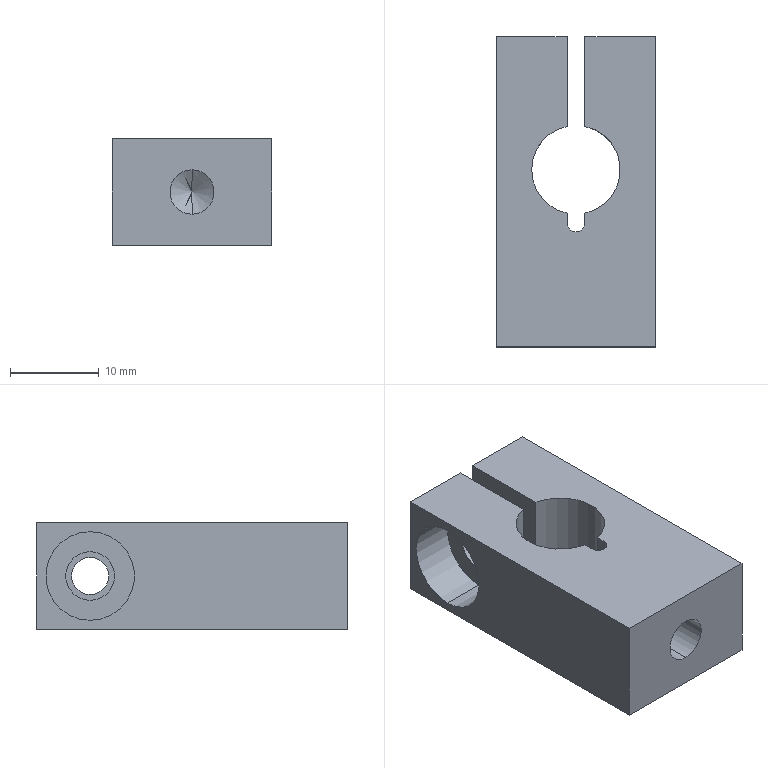Part | STEP file | Lock block wdl | 1 solid | 26 faces | box 18 x 35 x 12 mm | volume 5552 mm3 | cylinder 12 | plane 12 | cone 2 | commonest cylinder face diameters 10 x5 4.2 x2 5 x2 5.5 x2 2 x1
STEP:
#1=CARTESIAN_POINT('',(0.,-7.5,8.5));
#2=VERTEX_POINT('',#1);
#3=CARTESIAN_POINT('',(0.,-7.5,3.5));
#4=VERTEX_POINT('',#3);
#5=CARTESIAN_POINT('',(0.,-7.5,6.));
#6=DIRECTION('',(0.,-1.,0.));
#7=DIRECTION('',(0.,0.,-1.));
#8=AXIS2_PLACEMENT_3D('',#5,#6,#7);
#9=CIRCLE('',#8,2.5);
#10=EDGE_CURVE('',#2,#4,#9,.T.);
#11=ORIENTED_EDGE('',*,*,#10,.F.);
#12=CARTESIAN_POINT('',(0.,-17.5,8.5));
#13=VERTEX_POINT('',#12);
#14=CARTESIAN_POINT('',(0.,-17.5,8.5));
#15=DIRECTION('',(0.,-1.,0.));
#16=VECTOR('',#15,1000.);
#17=LINE('',#14,#16);
#18=EDGE_CURVE('',#2,#13,#17,.T.);
#19=ORIENTED_EDGE('',*,*,#18,.T.);
#20=CARTESIAN_POINT('',(0.,-17.5,3.5));
#21=VERTEX_POINT('',#20);
#22=CARTESIAN_POINT('',(0.,-17.5,6.));
#23=DIRECTION('',(0.,-1.,0.));
#24=DIRECTION('',(0.,0.,-1.));
#25=AXIS2_PLACEMENT_3D('',#22,#23,#24);
#26=CIRCLE('',#25,2.5);
#27=EDGE_CURVE('',#13,#21,#26,.T.);
#28=ORIENTED_EDGE('',*,*,#27,.T.);
#29=CARTESIAN_POINT('',(0.,-17.5,3.5));
#30=DIRECTION('',(0.,-1.,0.));
#31=VECTOR('',#30,1000.);
#32=LINE('',#29,#31);
#33=EDGE_CURVE('',#4,#21,#32,.T.);
#34=ORIENTED_EDGE('',*,*,#33,.F.);
#35=EDGE_LOOP('',(#11,#19,#28,#34));
#36=FACE_OUTER_BOUND('',#35,.T.);
#37=CARTESIAN_POINT('',(0.,-17.5,6.));
#38=DIRECTION('',(0.,-1.,0.));
#39=DIRECTION('',(0.,0.,-1.));
#40=AXIS2_PLACEMENT_3D('',#37,#38,#39);
#41=CYLINDRICAL_SURFACE('',#40,2.5);
#42=ADVANCED_FACE('',(#36),#41,.F.);
#43=CARTESIAN_POINT('',(0.,-5.998,6.));
#44=VERTEX_POINT('',#43);
#45=CARTESIAN_POINT('',(0.,-7.5,3.5));
#46=DIRECTION('',(0.,-0.515,-0.8572));
#47=VECTOR('',#46,1000.);
#48=LINE('',#45,#47);
#49=EDGE_CURVE('',#44,#4,#48,.T.);
#50=ORIENTED_EDGE('',*,*,#49,.F.);
#51=CARTESIAN_POINT('',(0.,-7.5,8.5));
#52=DIRECTION('',(0.,-0.515,0.8572));
#53=VECTOR('',#52,1000.);
#54=LINE('',#51,#53);
#55=EDGE_CURVE('',#44,#2,#54,.T.);
#56=ORIENTED_EDGE('',*,*,#55,.T.);
#57=ORIENTED_EDGE('',*,*,#10,.T.);
#58=EDGE_LOOP('',(#50,#56,#57));
#59=FACE_OUTER_BOUND('',#58,.T.);
#60=CARTESIAN_POINT('',(0.,-7.5,6.));
#61=DIRECTION('',(0.,-1.,0.));
#62=DIRECTION('',(0.,0.,-1.));
#63=AXIS2_PLACEMENT_3D('',#60,#61,#62);
#64=CONICAL_SURFACE('',#63,2.5,1.03);
#65=ADVANCED_FACE('',(#59),#64,.F.);
#66=CARTESIAN_POINT('',(9.,11.5,3.9));
#67=VERTEX_POINT('',#66);
#68=CARTESIAN_POINT('',(9.,11.5,8.1));
#69=VERTEX_POINT('',#68);
#70=CARTESIAN_POINT('',(9.,11.5,6.));
#71=DIRECTION('',(-1.,0.,0.));
#72=DIRECTION('',(0.,0.,1.));
#73=AXIS2_PLACEMENT_3D('',#70,#71,#72);
#74=CIRCLE('',#73,2.1);
#75=EDGE_CURVE('',#67,#69,#74,.T.);
#76=ORIENTED_EDGE('',*,*,#75,.F.);
#77=CARTESIAN_POINT('',(1.,11.5,3.9));
#78=VERTEX_POINT('',#77);
#79=CARTESIAN_POINT('',(1.,11.5,3.9));
#80=DIRECTION('',(-1.,0.,0.));
#81=VECTOR('',#80,1000.);
#82=LINE('',#79,#81);
#83=EDGE_CURVE('',#67,#78,#82,.T.);
#84=ORIENTED_EDGE('',*,*,#83,.T.);
#85=CARTESIAN_POINT('',(1.,11.5,8.1));
#86=VERTEX_POINT('',#85);
#87=CARTESIAN_POINT('',(1.,11.5,6.));
#88=DIRECTION('',(-1.,0.,0.));
#89=DIRECTION('',(0.,0.,1.));
#90=AXIS2_PLACEMENT_3D('',#87,#88,#89);
#91=CIRCLE('',#90,2.1);
#92=EDGE_CURVE('',#78,#86,#91,.T.);
#93=ORIENTED_EDGE('',*,*,#92,.T.);
#94=CARTESIAN_POINT('',(1.,11.5,8.1));
#95=DIRECTION('',(-1.,0.,0.));
#96=VECTOR('',#95,1000.);
#97=LINE('',#94,#96);
#98=EDGE_CURVE('',#69,#86,#97,.T.);
#99=ORIENTED_EDGE('',*,*,#98,.F.);
#100=EDGE_LOOP('',(#76,#84,#93,#99));
#101=FACE_OUTER_BOUND('',#100,.T.);
#102=CARTESIAN_POINT('',(1.,11.5,6.));
#103=DIRECTION('',(-1.,0.,0.));
#104=DIRECTION('',(0.,0.,1.));
#105=AXIS2_PLACEMENT_3D('',#102,#103,#104);
#106=CYLINDRICAL_SURFACE('',#105,2.1);
#107=ADVANCED_FACE('',(#101),#106,.F.);
#108=CARTESIAN_POINT('',(-4.,11.5,1.));
#109=VERTEX_POINT('',#108);
#110=CARTESIAN_POINT('',(-4.,11.5,11.));
#111=VERTEX_POINT('',#110);
#112=CARTESIAN_POINT('',(-4.,11.5,6.));
#113=DIRECTION('',(-1.,0.,0.));
#114=DIRECTION('',(0.,0.,1.));
#115=AXIS2_PLACEMENT_3D('',#112,#113,#114);
#116=CIRCLE('',#115,5.);
#117=EDGE_CURVE('',#109,#111,#116,.T.);
#118=ORIENTED_EDGE('',*,*,#117,.F.);
#119=CARTESIAN_POINT('',(-9.,11.5,1.));
#120=VERTEX_POINT('',#119);
#121=CARTESIAN_POINT('',(-9.,11.5,1.));
#122=DIRECTION('',(-1.,0.,0.));
#123=VECTOR('',#122,1000.);
#124=LINE('',#121,#123);
#125=EDGE_CURVE('',#109,#120,#124,.T.);
#126=ORIENTED_EDGE('',*,*,#125,.T.);
#127=CARTESIAN_POINT('',(-9.,11.5,11.));
#128=VERTEX_POINT('',#127);
#129=CARTESIAN_POINT('',(-9.,11.5,6.));
#130=DIRECTION('',(-1.,0.,0.));
#131=DIRECTION('',(0.,0.,1.));
#132=AXIS2_PLACEMENT_3D('',#129,#130,#131);
#133=CIRCLE('',#132,5.);
#134=EDGE_CURVE('',#120,#128,#133,.T.);
#135=ORIENTED_EDGE('',*,*,#134,.T.);
#136=CARTESIAN_POINT('',(-9.,11.5,11.));
#137=DIRECTION('',(-1.,0.,0.));
#138=VECTOR('',#137,1000.);
#139=LINE('',#136,#138);
#140=EDGE_CURVE('',#111,#128,#139,.T.);
#141=ORIENTED_EDGE('',*,*,#140,.F.);
#142=EDGE_LOOP('',(#118,#126,#135,#141));
#143=FACE_OUTER_BOUND('',#142,.T.);
#144=CARTESIAN_POINT('',(-9.,11.5,6.));
#145=DIRECTION('',(-1.,0.,0.));
#146=DIRECTION('',(0.,0.,1.));
#147=AXIS2_PLACEMENT_3D('',#144,#145,#146);
#148=CYLINDRICAL_SURFACE('',#147,5.);
#149=ADVANCED_FACE('',(#143),#148,.F.);
#150=CARTESIAN_POINT('',(-1.,11.5,3.25));
#151=VERTEX_POINT('',#150);
#152=CARTESIAN_POINT('',(-1.,11.5,8.75));
#153=VERTEX_POINT('',#152);
#154=CARTESIAN_POINT('',(-1.,11.5,6.));
#155=DIRECTION('',(-1.,0.,0.));
#156=DIRECTION('',(0.,-1.,0.));
#157=AXIS2_PLACEMENT_3D('',#154,#155,#156);
#158=CIRCLE('',#157,2.75);
#159=EDGE_CURVE('',#151,#153,#158,.T.);
#160=ORIENTED_EDGE('',*,*,#159,.F.);
#161=CARTESIAN_POINT('',(-4.,11.5,3.25));
#162=VERTEX_POINT('',#161);
#163=CARTESIAN_POINT('',(-9.,11.5,3.25));
#164=DIRECTION('',(-1.,0.,0.));
#165=VECTOR('',#164,1000.);
#166=LINE('',#163,#165);
#167=EDGE_CURVE('',#151,#162,#166,.T.);
#168=ORIENTED_EDGE('',*,*,#167,.T.);
#169=CARTESIAN_POINT('',(-4.,11.5,8.75));
#170=VERTEX_POINT('',#169);
#171=CARTESIAN_POINT('',(-4.,11.5,6.));
#172=DIRECTION('',(-1.,0.,0.));
#173=DIRECTION('',(0.,0.,1.));
#174=AXIS2_PLACEMENT_3D('',#171,#172,#173);
#175=CIRCLE('',#174,2.75);
#176=EDGE_CURVE('',#162,#170,#175,.T.);
#177=ORIENTED_EDGE('',*,*,#176,.T.);
#178=CARTESIAN_POINT('',(-9.,11.5,8.75));
#179=DIRECTION('',(-1.,0.,0.));
#180=VECTOR('',#179,1000.);
#181=LINE('',#178,#180);
#182=EDGE_CURVE('',#153,#170,#181,.T.);
#183=ORIENTED_EDGE('',*,*,#182,.F.);
#184=EDGE_LOOP('',(#160,#168,#177,#183));
#185=FACE_OUTER_BOUND('',#184,.T.);
#186=CARTESIAN_POINT('',(-9.,11.5,6.));
#187=DIRECTION('',(-1.,0.,0.));
#188=DIRECTION('',(0.,0.,1.));
#189=AXIS2_PLACEMENT_3D('',#186,#187,#188);
#190=CYLINDRICAL_SURFACE('',#189,2.75);
#191=ADVANCED_FACE('',(#185),#190,.F.);
#192=CARTESIAN_POINT('',(-1.,7.399,12.));
#193=VERTEX_POINT('',#192);
#194=CARTESIAN_POINT('',(-5.,2.5,12.));
#195=VERTEX_POINT('',#194);
#196=CARTESIAN_POINT('',(0.,2.5,12.));
#197=DIRECTION('',(0.,0.,1.));
#198=DIRECTION('',(1.,0.,0.));
#199=AXIS2_PLACEMENT_3D('',#196,#197,#198);
#200=CIRCLE('',#199,5.);
#201=EDGE_CURVE('',#193,#195,#200,.T.);
#202=ORIENTED_EDGE('',*,*,#201,.T.);
#203=CARTESIAN_POINT('',(-5.,2.5,0.));
#204=VERTEX_POINT('',#203);
#205=CARTESIAN_POINT('',(-5.,2.5,12.));
#206=DIRECTION('',(0.,0.,-1.));
#207=VECTOR('',#206,1000.);
#208=LINE('',#205,#207);
#209=EDGE_CURVE('',#195,#204,#208,.T.);
#210=ORIENTED_EDGE('',*,*,#209,.T.);
#211=CARTESIAN_POINT('',(-1.,7.399,0.));
#212=VERTEX_POINT('',#211);
#213=CARTESIAN_POINT('',(0.,2.5,0.));
#214=DIRECTION('',(0.,0.,1.));
#215=DIRECTION('',(1.,0.,0.));
#216=AXIS2_PLACEMENT_3D('',#213,#214,#215);
#217=CIRCLE('',#216,5.);
#218=EDGE_CURVE('',#212,#204,#217,.T.);
#219=ORIENTED_EDGE('',*,*,#218,.F.);
#220=CARTESIAN_POINT('',(-1.,7.399,12.));
#221=DIRECTION('',(0.,0.,-1.));
#222=VECTOR('',#221,1000.);
#223=LINE('',#220,#222);
#224=EDGE_CURVE('',#193,#212,#223,.T.);
#225=ORIENTED_EDGE('',*,*,#224,.F.);
#226=EDGE_LOOP('',(#202,#210,#219,#225));
#227=FACE_OUTER_BOUND('',#226,.T.);
#228=CARTESIAN_POINT('',(0.,2.5,12.));
#229=DIRECTION('',(0.,0.,-1.));
#230=DIRECTION('',(-1.,0.,0.));
#231=AXIS2_PLACEMENT_3D('',#228,#229,#230);
#232=CYLINDRICAL_SURFACE('',#231,5.);
#233=ADVANCED_FACE('',(#227),#232,.F.);
#234=CARTESIAN_POINT('',(9.,17.5,0.));
#235=VERTEX_POINT('',#234);
#236=CARTESIAN_POINT('',(1.,17.5,0.));
#237=VERTEX_POINT('',#236);
#238=CARTESIAN_POINT('',(-9.,17.5,0.));
#239=DIRECTION('',(-1.,0.,0.));
#240=VECTOR('',#239,1000.);
#241=LINE('',#238,#240);
#242=EDGE_CURVE('',#235,#237,#241,.T.);
#243=ORIENTED_EDGE('',*,*,#242,.T.);
#244=CARTESIAN_POINT('',(1.,17.5,12.));
#245=VERTEX_POINT('',#244);
#246=CARTESIAN_POINT('',(1.,17.5,0.));
#247=DIRECTION('',(0.,0.,1.));
#248=VECTOR('',#247,1000.);
#249=LINE('',#246,#248);
#250=EDGE_CURVE('',#237,#245,#249,.T.);
#251=ORIENTED_EDGE('',*,*,#250,.T.);
#252=CARTESIAN_POINT('',(9.,17.5,12.));
#253=VERTEX_POINT('',#252);
#254=CARTESIAN_POINT('',(-9.,17.5,12.));
#255=DIRECTION('',(-1.,0.,0.));
#256=VECTOR('',#255,1000.);
#257=LINE('',#254,#256);
#258=EDGE_CURVE('',#253,#245,#257,.T.);
#259=ORIENTED_EDGE('',*,*,#258,.F.);
#260=CARTESIAN_POINT('',(9.,17.5,12.));
#261=DIRECTION('',(0.,0.,-1.));
#262=VECTOR('',#261,1000.);
#263=LINE('',#260,#262);
#264=EDGE_CURVE('',#253,#235,#263,.T.);
#265=ORIENTED_EDGE('',*,*,#264,.T.);
#266=EDGE_LOOP('',(#243,#251,#259,#265));
#267=FACE_OUTER_BOUND('',#266,.T.);
#268=CARTESIAN_POINT('',(-9.,17.5,12.));
#269=DIRECTION('',(0.,-1.,0.));
#270=DIRECTION('',(0.,0.,-1.));
#271=AXIS2_PLACEMENT_3D('',#268,#269,#270);
#272=PLANE('',#271);
#273=ADVANCED_FACE('',(#267),#272,.F.);
#274=CARTESIAN_POINT('',(1.,-2.399,12.));
#275=VERTEX_POINT('',#274);
#276=CARTESIAN_POINT('',(1.,-2.399,0.));
#277=VERTEX_POINT('',#276);
#278=CARTESIAN_POINT('',(1.,-2.399,12.));
#279=DIRECTION('',(0.,0.,-1.));
#280=VECTOR('',#279,1000.);
#281=LINE('',#278,#280);
#282=EDGE_CURVE('',#275,#277,#281,.T.);
#283=ORIENTED_EDGE('',*,*,#282,.F.);
#284=CARTESIAN_POINT('',(1.,7.399,12.));
#285=VERTEX_POINT('',#284);
#286=CARTESIAN_POINT('',(0.,2.5,12.));
#287=DIRECTION('',(0.,0.,1.));
#288=DIRECTION('',(1.,0.,0.));
#289=AXIS2_PLACEMENT_3D('',#286,#287,#288);
#290=CIRCLE('',#289,5.);
#291=EDGE_CURVE('',#275,#285,#290,.T.);
#292=ORIENTED_EDGE('',*,*,#291,.T.);
#293=CARTESIAN_POINT('',(1.,7.399,0.));
#294=VERTEX_POINT('',#293);
#295=CARTESIAN_POINT('',(1.,7.399,12.));
#296=DIRECTION('',(0.,0.,1.));
#297=VECTOR('',#296,1000.);
#298=LINE('',#295,#297);
#299=EDGE_CURVE('',#294,#285,#298,.T.);
#300=ORIENTED_EDGE('',*,*,#299,.F.);
#301=CARTESIAN_POINT('',(0.,2.5,0.));
#302=DIRECTION('',(0.,0.,1.));
#303=DIRECTION('',(1.,0.,0.));
#304=AXIS2_PLACEMENT_3D('',#301,#302,#303);
#305=CIRCLE('',#304,5.);
#306=EDGE_CURVE('',#277,#294,#305,.T.);
#307=ORIENTED_EDGE('',*,*,#306,.F.);
#308=EDGE_LOOP('',(#283,#292,#300,#307));
#309=FACE_OUTER_BOUND('',#308,.T.);
#310=CARTESIAN_POINT('',(0.,2.5,12.));
#311=DIRECTION('',(0.,0.,-1.));
#312=DIRECTION('',(-1.,0.,0.));
#313=AXIS2_PLACEMENT_3D('',#310,#311,#312);
#314=CYLINDRICAL_SURFACE('',#313,5.);
#315=ADVANCED_FACE('',(#309),#314,.F.);
#316=ORIENTED_EDGE('',*,*,#258,.T.);
#317=CARTESIAN_POINT('',(1.,17.5,12.));
#318=DIRECTION('',(0.,1.,0.));
#319=VECTOR('',#318,1000.);
#320=LINE('',#317,#319);
#321=EDGE_CURVE('',#285,#245,#320,.T.);
#322=ORIENTED_EDGE('',*,*,#321,.F.);
#323=ORIENTED_EDGE('',*,*,#291,.F.);
#324=CARTESIAN_POINT('',(1.,-3.5,12.));
#325=VERTEX_POINT('',#324);
#326=CARTESIAN_POINT('',(1.,17.5,12.));
#327=DIRECTION('',(0.,1.,0.));
#328=VECTOR('',#327,1000.);
#329=LINE('',#326,#328);
#330=EDGE_CURVE('',#325,#275,#329,.T.);
#331=ORIENTED_EDGE('',*,*,#330,.F.);
#332=CARTESIAN_POINT('',(-1.,-3.5,12.));
#333=VERTEX_POINT('',#332);
#334=CARTESIAN_POINT('',(0.,-3.5,12.));
#335=DIRECTION('',(0.,0.,1.));
#336=DIRECTION('',(1.,0.,0.));
#337=AXIS2_PLACEMENT_3D('',#334,#335,#336);
#338=CIRCLE('',#337,1.);
#339=EDGE_CURVE('',#333,#325,#338,.T.);
#340=ORIENTED_EDGE('',*,*,#339,.F.);
#341=CARTESIAN_POINT('',(-1.,-2.399,12.));
#342=VERTEX_POINT('',#341);
#343=CARTESIAN_POINT('',(-1.,17.5,12.));
#344=DIRECTION('',(0.,-1.,0.));
#345=VECTOR('',#344,1000.);
#346=LINE('',#343,#345);
#347=EDGE_CURVE('',#342,#333,#346,.T.);
#348=ORIENTED_EDGE('',*,*,#347,.F.);
#349=CARTESIAN_POINT('',(0.,2.5,12.));
#350=DIRECTION('',(0.,0.,1.));
#351=DIRECTION('',(1.,0.,0.));
#352=AXIS2_PLACEMENT_3D('',#349,#350,#351);
#353=CIRCLE('',#352,5.);
#354=EDGE_CURVE('',#195,#342,#353,.T.);
#355=ORIENTED_EDGE('',*,*,#354,.F.);
#356=ORIENTED_EDGE('',*,*,#201,.F.);
#357=CARTESIAN_POINT('',(-1.,17.5,12.));
#358=VERTEX_POINT('',#357);
#359=CARTESIAN_POINT('',(-1.,17.5,12.));
#360=DIRECTION('',(0.,-1.,0.));
#361=VECTOR('',#360,1000.);
#362=LINE('',#359,#361);
#363=EDGE_CURVE('',#358,#193,#362,.T.);
#364=ORIENTED_EDGE('',*,*,#363,.F.);
#365=CARTESIAN_POINT('',(-9.,17.5,12.));
#366=VERTEX_POINT('',#365);
#367=CARTESIAN_POINT('',(-9.,17.5,12.));
#368=DIRECTION('',(-1.,0.,0.));
#369=VECTOR('',#368,1000.);
#370=LINE('',#367,#369);
#371=EDGE_CURVE('',#358,#366,#370,.T.);
#372=ORIENTED_EDGE('',*,*,#371,.T.);
#373=CARTESIAN_POINT('',(-9.,-17.5,12.));
#374=VERTEX_POINT('',#373);
#375=CARTESIAN_POINT('',(-9.,-17.5,12.));
#376=DIRECTION('',(0.,-1.,0.));
#377=VECTOR('',#376,1000.);
#378=LINE('',#375,#377);
#379=EDGE_CURVE('',#366,#374,#378,.T.);
#380=ORIENTED_EDGE('',*,*,#379,.T.);
#381=CARTESIAN_POINT('',(9.,-17.5,12.));
#382=VERTEX_POINT('',#381);
#383=CARTESIAN_POINT('',(-9.,-17.5,12.));
#384=DIRECTION('',(1.,0.,0.));
#385=VECTOR('',#384,1000.);
#386=LINE('',#383,#385);
#387=EDGE_CURVE('',#374,#382,#386,.T.);
#388=ORIENTED_EDGE('',*,*,#387,.T.);
#389=CARTESIAN_POINT('',(9.,-17.5,12.));
#390=DIRECTION('',(0.,1.,0.));
#391=VECTOR('',#390,1000.);
#392=LINE('',#389,#391);
#393=EDGE_CURVE('',#382,#253,#392,.T.);
#394=ORIENTED_EDGE('',*,*,#393,.T.);
#395=EDGE_LOOP('',(#316,#322,#323,#331,#340,#348,#355,#356,#364,#372,#380,#388,#394));
#396=FACE_OUTER_BOUND('',#395,.T.);
#397=CARTESIAN_POINT('',(9.,17.5,12.));
#398=DIRECTION('',(0.,0.,-1.));
#399=DIRECTION('',(-1.,0.,0.));
#400=AXIS2_PLACEMENT_3D('',#397,#398,#399);
#401=PLANE('',#400);
#402=ADVANCED_FACE('',(#396),#401,.F.);
#403=CARTESIAN_POINT('',(1.,17.5,0.));
#404=DIRECTION('',(0.,1.,0.));
#405=VECTOR('',#404,1000.);
#406=LINE('',#403,#405);
#407=EDGE_CURVE('',#294,#237,#406,.T.);
#408=ORIENTED_EDGE('',*,*,#407,.T.);
#409=ORIENTED_EDGE('',*,*,#242,.F.);
#410=CARTESIAN_POINT('',(9.,-17.5,0.));
#411=VERTEX_POINT('',#410);
#412=CARTESIAN_POINT('',(9.,-17.5,0.));
#413=DIRECTION('',(0.,1.,0.));
#414=VECTOR('',#413,1000.);
#415=LINE('',#412,#414);
#416=EDGE_CURVE('',#411,#235,#415,.T.);
#417=ORIENTED_EDGE('',*,*,#416,.F.);
#418=CARTESIAN_POINT('',(-9.,-17.5,0.));
#419=VERTEX_POINT('',#418);
#420=CARTESIAN_POINT('',(-9.,-17.5,0.));
#421=DIRECTION('',(1.,0.,0.));
#422=VECTOR('',#421,1000.);
#423=LINE('',#420,#422);
#424=EDGE_CURVE('',#419,#411,#423,.T.);
#425=ORIENTED_EDGE('',*,*,#424,.F.);
#426=CARTESIAN_POINT('',(-9.,17.5,0.));
#427=VERTEX_POINT('',#426);
#428=CARTESIAN_POINT('',(-9.,-17.5,0.));
#429=DIRECTION('',(0.,-1.,0.));
#430=VECTOR('',#429,1000.);
#431=LINE('',#428,#430);
#432=EDGE_CURVE('',#427,#419,#431,.T.);
#433=ORIENTED_EDGE('',*,*,#432,.F.);
#434=CARTESIAN_POINT('',(-1.,17.5,0.));
#435=VERTEX_POINT('',#434);
#436=CARTESIAN_POINT('',(-9.,17.5,0.));
#437=DIRECTION('',(-1.,0.,0.));
#438=VECTOR('',#437,1000.);
#439=LINE('',#436,#438);
#440=EDGE_CURVE('',#435,#427,#439,.T.);
#441=ORIENTED_EDGE('',*,*,#440,.F.);
#442=CARTESIAN_POINT('',(-1.,17.5,0.));
#443=DIRECTION('',(0.,-1.,0.));
#444=VECTOR('',#443,1000.);
#445=LINE('',#442,#444);
#446=EDGE_CURVE('',#435,#212,#445,.T.);
#447=ORIENTED_EDGE('',*,*,#446,.T.);
#448=ORIENTED_EDGE('',*,*,#218,.T.);
#449=CARTESIAN_POINT('',(-1.,-2.399,0.));
#450=VERTEX_POINT('',#449);
#451=CARTESIAN_POINT('',(0.,2.5,0.));
#452=DIRECTION('',(0.,0.,1.));
#453=DIRECTION('',(1.,0.,0.));
#454=AXIS2_PLACEMENT_3D('',#451,#452,#453);
#455=CIRCLE('',#454,5.);
#456=EDGE_CURVE('',#204,#450,#455,.T.);
#457=ORIENTED_EDGE('',*,*,#456,.T.);
#458=CARTESIAN_POINT('',(-1.,-3.5,0.));
#459=VERTEX_POINT('',#458);
#460=CARTESIAN_POINT('',(-1.,17.5,0.));
#461=DIRECTION('',(0.,-1.,0.));
#462=VECTOR('',#461,1000.);
#463=LINE('',#460,#462);
#464=EDGE_CURVE('',#450,#459,#463,.T.);
#465=ORIENTED_EDGE('',*,*,#464,.T.);
#466=CARTESIAN_POINT('',(1.,-3.5,0.));
#467=VERTEX_POINT('',#466);
#468=CARTESIAN_POINT('',(0.,-3.5,0.));
#469=DIRECTION('',(0.,0.,1.));
#470=DIRECTION('',(1.,0.,0.));
#471=AXIS2_PLACEMENT_3D('',#468,#469,#470);
#472=CIRCLE('',#471,1.);
#473=EDGE_CURVE('',#459,#467,#472,.T.);
#474=ORIENTED_EDGE('',*,*,#473,.T.);
#475=CARTESIAN_POINT('',(1.,17.5,0.));
#476=DIRECTION('',(0.,1.,0.));
#477=VECTOR('',#476,1000.);
#478=LINE('',#475,#477);
#479=EDGE_CURVE('',#467,#277,#478,.T.);
#480=ORIENTED_EDGE('',*,*,#479,.T.);
#481=ORIENTED_EDGE('',*,*,#306,.T.);
#482=EDGE_LOOP('',(#408,#409,#417,#425,#433,#441,#447,#448,#457,#465,#474,#480,#481));
#483=FACE_OUTER_BOUND('',#482,.T.);
#484=CARTESIAN_POINT('',(9.,17.5,0.));
#485=DIRECTION('',(0.,0.,-1.));
#486=DIRECTION('',(-1.,0.,0.));
#487=AXIS2_PLACEMENT_3D('',#484,#485,#486);
#488=PLANE('',#487);
#489=ADVANCED_FACE('',(#483),#488,.T.);
#490=CARTESIAN_POINT('',(9.,11.5,6.));
#491=DIRECTION('',(-1.,0.,0.));
#492=DIRECTION('',(0.,0.,1.));
#493=AXIS2_PLACEMENT_3D('',#490,#491,#492);
#494=CIRCLE('',#493,2.1);
#495=EDGE_CURVE('',#69,#67,#494,.T.);
#496=ORIENTED_EDGE('',*,*,#495,.T.);
#497=ORIENTED_EDGE('',*,*,#75,.T.);
#498=EDGE_LOOP('',(#496,#497));
#499=FACE_BOUND('',#498,.T.);
#500=ORIENTED_EDGE('',*,*,#416,.T.);
#501=ORIENTED_EDGE('',*,*,#264,.F.);
#502=ORIENTED_EDGE('',*,*,#393,.F.);
#503=CARTESIAN_POINT('',(9.,-17.5,12.));
#504=DIRECTION('',(0.,0.,-1.));
#505=VECTOR('',#504,1000.);
#506=LINE('',#503,#505);
#507=EDGE_CURVE('',#382,#411,#506,.T.);
#508=ORIENTED_EDGE('',*,*,#507,.T.);
#509=EDGE_LOOP('',(#500,#501,#502,#508));
#510=FACE_OUTER_BOUND('',#509,.T.);
#511=CARTESIAN_POINT('',(9.,-17.5,12.));
#512=DIRECTION('',(-1.,0.,0.));
#513=DIRECTION('',(0.,0.,1.));
#514=AXIS2_PLACEMENT_3D('',#511,#512,#513);
#515=PLANE('',#514);
#516=ADVANCED_FACE('',(#499,#510),#515,.F.);
#517=ORIENTED_EDGE('',*,*,#371,.F.);
#518=CARTESIAN_POINT('',(-1.,17.5,0.));
#519=DIRECTION('',(0.,0.,1.));
#520=VECTOR('',#519,1000.);
#521=LINE('',#518,#520);
#522=EDGE_CURVE('',#435,#358,#521,.T.);
#523=ORIENTED_EDGE('',*,*,#522,.F.);
#524=ORIENTED_EDGE('',*,*,#440,.T.);
#525=CARTESIAN_POINT('',(-9.,17.5,12.));
#526=DIRECTION('',(0.,0.,-1.));
#527=VECTOR('',#526,1000.);
#528=LINE('',#525,#527);
#529=EDGE_CURVE('',#366,#427,#528,.T.);
#530=ORIENTED_EDGE('',*,*,#529,.F.);
#531=EDGE_LOOP('',(#517,#523,#524,#530));
#532=FACE_OUTER_BOUND('',#531,.T.);
#533=CARTESIAN_POINT('',(-9.,17.5,12.));
#534=DIRECTION('',(0.,-1.,0.));
#535=DIRECTION('',(0.,0.,-1.));
#536=AXIS2_PLACEMENT_3D('',#533,#534,#535);
#537=PLANE('',#536);
#538=ADVANCED_FACE('',(#532),#537,.F.);
#539=CARTESIAN_POINT('',(-9.,11.5,6.));
#540=DIRECTION('',(-1.,0.,0.));
#541=DIRECTION('',(0.,0.,1.));
#542=AXIS2_PLACEMENT_3D('',#539,#540,#541);
#543=CIRCLE('',#542,5.);
#544=EDGE_CURVE('',#128,#120,#543,.T.);
#545=ORIENTED_EDGE('',*,*,#544,.F.);
#546=ORIENTED_EDGE('',*,*,#134,.F.);
#547=EDGE_LOOP('',(#545,#546));
#548=FACE_BOUND('',#547,.T.);
#549=ORIENTED_EDGE('',*,*,#432,.T.);
#550=CARTESIAN_POINT('',(-9.,-17.5,12.));
#551=DIRECTION('',(0.,0.,-1.));
#552=VECTOR('',#551,1000.);
#553=LINE('',#550,#552);
#554=EDGE_CURVE('',#374,#419,#553,.T.);
#555=ORIENTED_EDGE('',*,*,#554,.F.);
#556=ORIENTED_EDGE('',*,*,#379,.F.);
#557=ORIENTED_EDGE('',*,*,#529,.T.);
#558=EDGE_LOOP('',(#549,#555,#556,#557));
#559=FACE_OUTER_BOUND('',#558,.T.);
#560=CARTESIAN_POINT('',(-9.,-17.5,12.));
#561=DIRECTION('',(1.,0.,0.));
#562=DIRECTION('',(0.,0.,-1.));
#563=AXIS2_PLACEMENT_3D('',#560,#561,#562);
#564=PLANE('',#563);
#565=ADVANCED_FACE('',(#548,#559),#564,.F.);
#566=CARTESIAN_POINT('',(0.,-17.5,6.));
#567=DIRECTION('',(0.,-1.,0.));
#568=DIRECTION('',(0.,0.,-1.));
#569=AXIS2_PLACEMENT_3D('',#566,#567,#568);
#570=CIRCLE('',#569,2.5);
#571=EDGE_CURVE('',#21,#13,#570,.T.);
#572=ORIENTED_EDGE('',*,*,#571,.F.);
#573=ORIENTED_EDGE('',*,*,#27,.F.);
#574=EDGE_LOOP('',(#572,#573));
#575=FACE_BOUND('',#574,.T.);
#576=ORIENTED_EDGE('',*,*,#424,.T.);
#577=ORIENTED_EDGE('',*,*,#507,.F.);
#578=ORIENTED_EDGE('',*,*,#387,.F.);
#579=ORIENTED_EDGE('',*,*,#554,.T.);
#580=EDGE_LOOP('',(#576,#577,#578,#579));
#581=FACE_OUTER_BOUND('',#580,.T.);
#582=CARTESIAN_POINT('',(-9.,-17.5,12.));
#583=DIRECTION('',(0.,1.,0.));
#584=DIRECTION('',(0.,0.,1.));
#585=AXIS2_PLACEMENT_3D('',#582,#583,#584);
#586=PLANE('',#585);
#587=ADVANCED_FACE('',(#575,#581),#586,.F.);
#588=ORIENTED_EDGE('',*,*,#209,.F.);
#589=ORIENTED_EDGE('',*,*,#354,.T.);
#590=CARTESIAN_POINT('',(-1.,-2.399,12.));
#591=DIRECTION('',(0.,0.,1.));
#592=VECTOR('',#591,1000.);
#593=LINE('',#590,#592);
#594=EDGE_CURVE('',#450,#342,#593,.T.);
#595=ORIENTED_EDGE('',*,*,#594,.F.);
#596=ORIENTED_EDGE('',*,*,#456,.F.);
#597=EDGE_LOOP('',(#588,#589,#595,#596));
#598=FACE_OUTER_BOUND('',#597,.T.);
#599=CARTESIAN_POINT('',(0.,2.5,12.));
#600=DIRECTION('',(0.,0.,-1.));
#601=DIRECTION('',(-1.,0.,0.));
#602=AXIS2_PLACEMENT_3D('',#599,#600,#601);
#603=CYLINDRICAL_SURFACE('',#602,5.);
#604=ADVANCED_FACE('',(#598),#603,.F.);
#605=ORIENTED_EDGE('',*,*,#282,.T.);
#606=ORIENTED_EDGE('',*,*,#479,.F.);
#607=CARTESIAN_POINT('',(1.,-3.5,0.));
#608=DIRECTION('',(0.,0.,1.));
#609=VECTOR('',#608,1000.);
#610=LINE('',#607,#609);
#611=EDGE_CURVE('',#467,#325,#610,.T.);
#612=ORIENTED_EDGE('',*,*,#611,.T.);
#613=ORIENTED_EDGE('',*,*,#330,.T.);
#614=EDGE_LOOP('',(#605,#606,#612,#613));
#615=FACE_OUTER_BOUND('',#614,.T.);
#616=CARTESIAN_POINT('',(1.,17.5,0.));
#617=DIRECTION('',(1.,0.,0.));
#618=DIRECTION('',(0.,1.,0.));
#619=AXIS2_PLACEMENT_3D('',#616,#617,#618);
#620=PLANE('',#619);
#621=ADVANCED_FACE('',(#615),#620,.F.);
#622=ORIENTED_EDGE('',*,*,#594,.T.);
#623=ORIENTED_EDGE('',*,*,#347,.T.);
#624=CARTESIAN_POINT('',(-1.,-3.5,0.));
#625=DIRECTION('',(0.,0.,1.));
#626=VECTOR('',#625,1000.);
#627=LINE('',#624,#626);
#628=EDGE_CURVE('',#459,#333,#627,.T.);
#629=ORIENTED_EDGE('',*,*,#628,.F.);
#630=ORIENTED_EDGE('',*,*,#464,.F.);
#631=EDGE_LOOP('',(#622,#623,#629,#630));
#632=FACE_OUTER_BOUND('',#631,.T.);
#633=CARTESIAN_POINT('',(-1.,17.5,0.));
#634=DIRECTION('',(-1.,0.,0.));
#635=DIRECTION('',(0.,-1.,0.));
#636=AXIS2_PLACEMENT_3D('',#633,#634,#635);
#637=PLANE('',#636);
#638=ADVANCED_FACE('',(#632),#637,.F.);
#639=ORIENTED_EDGE('',*,*,#339,.T.);
#640=ORIENTED_EDGE('',*,*,#611,.F.);
#641=ORIENTED_EDGE('',*,*,#473,.F.);
#642=ORIENTED_EDGE('',*,*,#628,.T.);
#643=EDGE_LOOP('',(#639,#640,#641,#642));
#644=FACE_OUTER_BOUND('',#643,.T.);
#645=CARTESIAN_POINT('',(0.,-3.5,0.));
#646=DIRECTION('',(0.,0.,1.));
#647=DIRECTION('',(1.,0.,0.));
#648=AXIS2_PLACEMENT_3D('',#645,#646,#647);
#649=CYLINDRICAL_SURFACE('',#648,1.);
#650=ADVANCED_FACE('',(#644),#649,.F.);
#651=CARTESIAN_POINT('',(-1.,11.5,6.));
#652=DIRECTION('',(-1.,0.,0.));
#653=DIRECTION('',(0.,-1.,0.));
#654=AXIS2_PLACEMENT_3D('',#651,#652,#653);
#655=CIRCLE('',#654,2.75);
#656=EDGE_CURVE('',#153,#151,#655,.T.);
#657=ORIENTED_EDGE('',*,*,#656,.T.);
#658=ORIENTED_EDGE('',*,*,#159,.T.);
#659=EDGE_LOOP('',(#657,#658));
#660=FACE_BOUND('',#659,.T.);
#661=ORIENTED_EDGE('',*,*,#224,.T.);
#662=ORIENTED_EDGE('',*,*,#446,.F.);
#663=ORIENTED_EDGE('',*,*,#522,.T.);
#664=ORIENTED_EDGE('',*,*,#363,.T.);
#665=EDGE_LOOP('',(#661,#662,#663,#664));
#666=FACE_OUTER_BOUND('',#665,.T.);
#667=CARTESIAN_POINT('',(-1.,17.5,0.));
#668=DIRECTION('',(-1.,0.,0.));
#669=DIRECTION('',(0.,-1.,0.));
#670=AXIS2_PLACEMENT_3D('',#667,#668,#669);
#671=PLANE('',#670);
#672=ADVANCED_FACE('',(#660,#666),#671,.F.);
#673=CARTESIAN_POINT('',(1.,11.5,6.));
#674=DIRECTION('',(-1.,0.,0.));
#675=DIRECTION('',(0.,0.,1.));
#676=AXIS2_PLACEMENT_3D('',#673,#674,#675);
#677=CIRCLE('',#676,2.1);
#678=EDGE_CURVE('',#86,#78,#677,.T.);
#679=ORIENTED_EDGE('',*,*,#678,.F.);
#680=ORIENTED_EDGE('',*,*,#92,.F.);
#681=EDGE_LOOP('',(#679,#680));
#682=FACE_BOUND('',#681,.T.);
#683=ORIENTED_EDGE('',*,*,#299,.T.);
#684=ORIENTED_EDGE('',*,*,#321,.T.);
#685=ORIENTED_EDGE('',*,*,#250,.F.);
#686=ORIENTED_EDGE('',*,*,#407,.F.);
#687=EDGE_LOOP('',(#683,#684,#685,#686));
#688=FACE_OUTER_BOUND('',#687,.T.);
#689=CARTESIAN_POINT('',(1.,17.5,0.));
#690=DIRECTION('',(1.,0.,0.));
#691=DIRECTION('',(0.,1.,0.));
#692=AXIS2_PLACEMENT_3D('',#689,#690,#691);
#693=PLANE('',#692);
#694=ADVANCED_FACE('',(#682,#688),#693,.F.);
#695=ORIENTED_EDGE('',*,*,#167,.F.);
#696=ORIENTED_EDGE('',*,*,#656,.F.);
#697=ORIENTED_EDGE('',*,*,#182,.T.);
#698=CARTESIAN_POINT('',(-4.,11.5,6.));
#699=DIRECTION('',(-1.,0.,0.));
#700=DIRECTION('',(0.,0.,1.));
#701=AXIS2_PLACEMENT_3D('',#698,#699,#700);
#702=CIRCLE('',#701,2.75);
#703=EDGE_CURVE('',#170,#162,#702,.T.);
#704=ORIENTED_EDGE('',*,*,#703,.T.);
#705=EDGE_LOOP('',(#695,#696,#697,#704));
#706=FACE_OUTER_BOUND('',#705,.T.);
#707=CARTESIAN_POINT('',(-9.,11.5,6.));
#708=DIRECTION('',(-1.,0.,0.));
#709=DIRECTION('',(0.,0.,1.));
#710=AXIS2_PLACEMENT_3D('',#707,#708,#709);
#711=CYLINDRICAL_SURFACE('',#710,2.75);
#712=ADVANCED_FACE('',(#706),#711,.F.);
#713=ORIENTED_EDGE('',*,*,#703,.F.);
#714=ORIENTED_EDGE('',*,*,#176,.F.);
#715=EDGE_LOOP('',(#713,#714));
#716=FACE_BOUND('',#715,.T.);
#717=CARTESIAN_POINT('',(-4.,11.5,6.));
#718=DIRECTION('',(-1.,0.,0.));
#719=DIRECTION('',(0.,0.,1.));
#720=AXIS2_PLACEMENT_3D('',#717,#718,#719);
#721=CIRCLE('',#720,5.);
#722=EDGE_CURVE('',#111,#109,#721,.T.);
#723=ORIENTED_EDGE('',*,*,#722,.T.);
#724=ORIENTED_EDGE('',*,*,#117,.T.);
#725=EDGE_LOOP('',(#723,#724));
#726=FACE_OUTER_BOUND('',#725,.T.);
#727=CARTESIAN_POINT('',(-4.,14.25,6.));
#728=DIRECTION('',(1.,0.,0.));
#729=DIRECTION('',(0.,0.,-1.));
#730=AXIS2_PLACEMENT_3D('',#727,#728,#729);
#731=PLANE('',#730);
#732=ADVANCED_FACE('',(#716,#726),#731,.F.);
#733=ORIENTED_EDGE('',*,*,#125,.F.);
#734=ORIENTED_EDGE('',*,*,#722,.F.);
#735=ORIENTED_EDGE('',*,*,#140,.T.);
#736=ORIENTED_EDGE('',*,*,#544,.T.);
#737=EDGE_LOOP('',(#733,#734,#735,#736));
#738=FACE_OUTER_BOUND('',#737,.T.);
#739=CARTESIAN_POINT('',(-9.,11.5,6.));
#740=DIRECTION('',(-1.,0.,0.));
#741=DIRECTION('',(0.,0.,1.));
#742=AXIS2_PLACEMENT_3D('',#739,#740,#741);
#743=CYLINDRICAL_SURFACE('',#742,5.);
#744=ADVANCED_FACE('',(#738),#743,.F.);
#745=ORIENTED_EDGE('',*,*,#83,.F.);
#746=ORIENTED_EDGE('',*,*,#495,.F.);
#747=ORIENTED_EDGE('',*,*,#98,.T.);
#748=ORIENTED_EDGE('',*,*,#678,.T.);
#749=EDGE_LOOP('',(#745,#746,#747,#748));
#750=FACE_OUTER_BOUND('',#749,.T.);
#751=CARTESIAN_POINT('',(1.,11.5,6.));
#752=DIRECTION('',(-1.,0.,0.));
#753=DIRECTION('',(0.,0.,1.));
#754=AXIS2_PLACEMENT_3D('',#751,#752,#753);
#755=CYLINDRICAL_SURFACE('',#754,2.1);
#756=ADVANCED_FACE('',(#750),#755,.F.);
#757=ORIENTED_EDGE('',*,*,#55,.F.);
#758=ORIENTED_EDGE('',*,*,#49,.T.);
#759=CARTESIAN_POINT('',(0.,-7.5,6.));
#760=DIRECTION('',(0.,-1.,0.));
#761=DIRECTION('',(0.,0.,-1.));
#762=AXIS2_PLACEMENT_3D('',#759,#760,#761);
#763=CIRCLE('',#762,2.5);
#764=EDGE_CURVE('',#4,#2,#763,.T.);
#765=ORIENTED_EDGE('',*,*,#764,.T.);
#766=EDGE_LOOP('',(#757,#758,#765));
#767=FACE_OUTER_BOUND('',#766,.T.);
#768=CARTESIAN_POINT('',(0.,-7.5,6.));
#769=DIRECTION('',(0.,-1.,0.));
#770=DIRECTION('',(0.,0.,-1.));
#771=AXIS2_PLACEMENT_3D('',#768,#769,#770);
#772=CONICAL_SURFACE('',#771,2.5,1.03);
#773=ADVANCED_FACE('',(#767),#772,.F.);
#774=ORIENTED_EDGE('',*,*,#18,.F.);
#775=ORIENTED_EDGE('',*,*,#764,.F.);
#776=ORIENTED_EDGE('',*,*,#33,.T.);
#777=ORIENTED_EDGE('',*,*,#571,.T.);
#778=EDGE_LOOP('',(#774,#775,#776,#777));
#779=FACE_OUTER_BOUND('',#778,.T.);
#780=CARTESIAN_POINT('',(0.,-17.5,6.));
#781=DIRECTION('',(0.,-1.,0.));
#782=DIRECTION('',(0.,0.,-1.));
#783=AXIS2_PLACEMENT_3D('',#780,#781,#782);
#784=CYLINDRICAL_SURFACE('',#783,2.5);
#785=ADVANCED_FACE('',(#779),#784,.F.);
#786=CLOSED_SHELL('',(#42,#65,#107,#149,#191,#233,#273,#315,#402,#489,#516,#538,#565,#587,#604,#621,#638,#650,#672,#694,#712,#732,#744,#756,#773,#785));
#787=MANIFOLD_SOLID_BREP('',#786);
#788=CARTESIAN_POINT('',(0.,0.,0.));
#789=DIRECTION('',(0.,0.,1.));
#790=DIRECTION('',(1.,0.,0.));
#791=AXIS2_PLACEMENT_3D('',#788,#789,#790);
#792=(LENGTH_UNIT()NAMED_UNIT(*)SI_UNIT(.MILLI.,.METRE.));
#793=UNCERTAINTY_MEASURE_WITH_UNIT(LENGTH_MEASURE(0.00001),#792,'','');
#794=(NAMED_UNIT(*)PLANE_ANGLE_UNIT()SI_UNIT($,.RADIAN.));
#795=(NAMED_UNIT(*)SI_UNIT($,.STERADIAN.)SOLID_ANGLE_UNIT());
#796=(GEOMETRIC_REPRESENTATION_CONTEXT(3)GLOBAL_UNCERTAINTY_ASSIGNED_CONTEXT((#793))GLOBAL_UNIT_ASSIGNED_CONTEXT((#792,#794,#795))REPRESENTATION_CONTEXT('',''));
#797=ADVANCED_BREP_SHAPE_REPRESENTATION('',(#787,#791),#796);